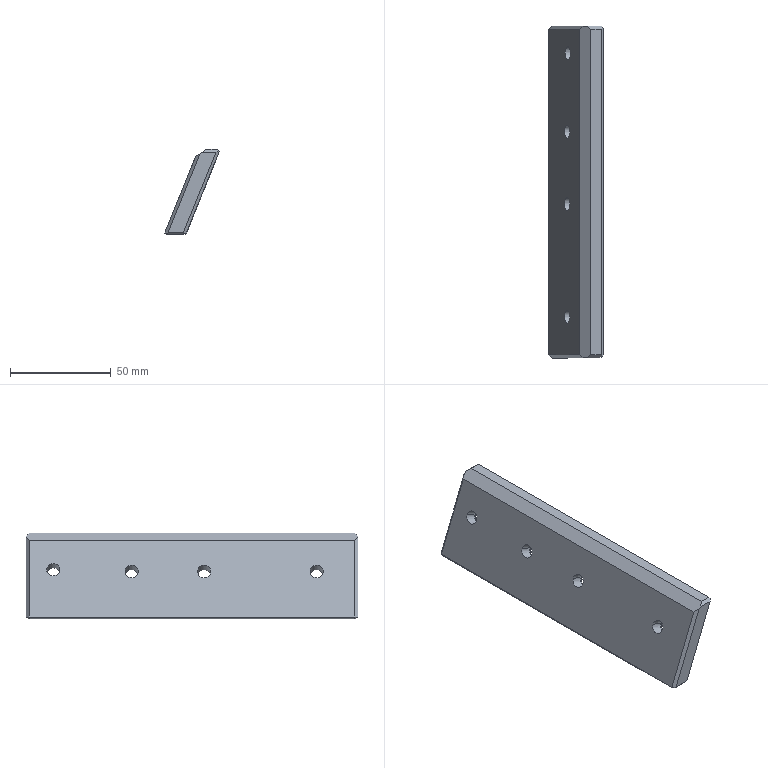Part | Creo | 1 solid | 46 faces | box 27.105 x 165 x 42.7 mm | volume 71949 mm3 | plane 22 | cylinder 16 | cone 8 | commonest cylinder face diameters 6.6 x8 13 x8